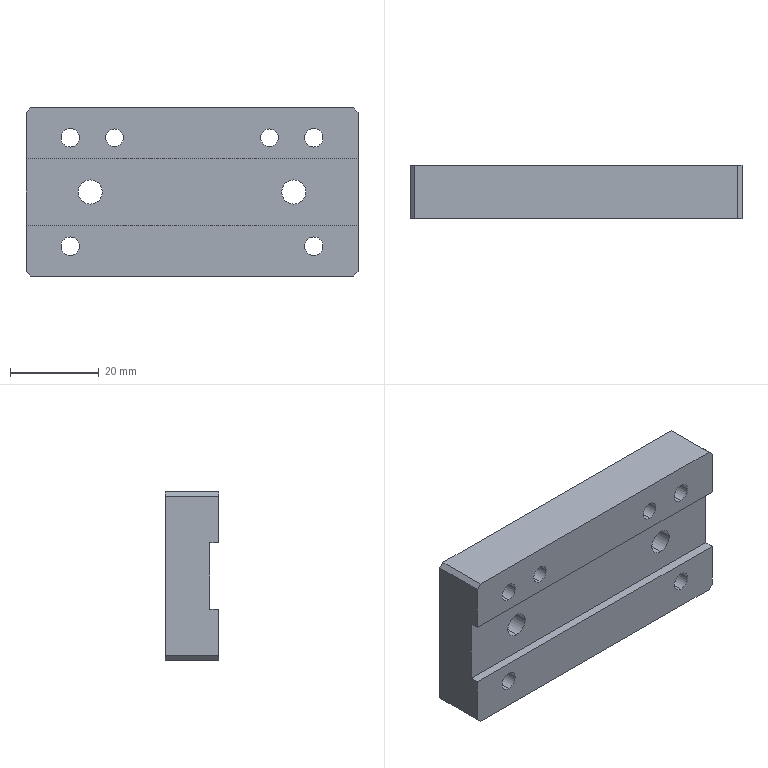Part | STEP file | 10000020593swp000-1 | 1 solid | 40 faces | box 75 x 12 x 38 mm | volume 29849 mm3 | cylinder 20 | plane 16 | cone 4 | commonest cylinder face diameters 4.2 x8 4 x4 5.5 x4 10 x4
STEP:
#1=CARTESIAN_POINT('',(-17.5,11.5,10.25));
#2=VERTEX_POINT('',#1);
#3=CARTESIAN_POINT('',(-17.5,11.5,14.25));
#4=VERTEX_POINT('',#3);
#5=CARTESIAN_POINT('',(-17.5,11.5,12.25));
#6=DIRECTION('',(0.,1.,0.));
#7=DIRECTION('',(0.,0.,1.));
#8=AXIS2_PLACEMENT_3D('',#5,#6,#7);
#9=CIRCLE('',#8,2.);
#10=EDGE_CURVE('',#2,#4,#9,.T.);
#11=ORIENTED_EDGE('',*,*,#10,.F.);
#12=CARTESIAN_POINT('',(-17.5,12.,9.75));
#13=VERTEX_POINT('',#12);
#14=CARTESIAN_POINT('',(-17.5,11.5,10.25));
#15=DIRECTION('',(0.,0.7071,-0.7071));
#16=VECTOR('',#15,1000.);
#17=LINE('',#14,#16);
#18=EDGE_CURVE('',#2,#13,#17,.T.);
#19=ORIENTED_EDGE('',*,*,#18,.T.);
#20=CARTESIAN_POINT('',(-17.5,12.,14.75));
#21=VERTEX_POINT('',#20);
#22=CARTESIAN_POINT('',(-17.5,12.,12.25));
#23=DIRECTION('',(0.,-1.,0.));
#24=DIRECTION('',(0.,0.,1.));
#25=AXIS2_PLACEMENT_3D('',#22,#23,#24);
#26=CIRCLE('',#25,2.5);
#27=EDGE_CURVE('',#21,#13,#26,.T.);
#28=ORIENTED_EDGE('',*,*,#27,.F.);
#29=CARTESIAN_POINT('',(-17.5,11.5,14.25));
#30=DIRECTION('',(0.,0.7071,0.7071));
#31=VECTOR('',#30,1000.);
#32=LINE('',#29,#31);
#33=EDGE_CURVE('',#4,#21,#32,.T.);
#34=ORIENTED_EDGE('',*,*,#33,.F.);
#35=EDGE_LOOP('',(#11,#19,#28,#34));
#36=FACE_OUTER_BOUND('',#35,.T.);
#37=CARTESIAN_POINT('',(-17.5,11.5,12.25));
#38=DIRECTION('',(0.,1.,0.));
#39=DIRECTION('',(0.,0.,1.));
#40=AXIS2_PLACEMENT_3D('',#37,#38,#39);
#41=CONICAL_SURFACE('',#40,2.,0.7854);
#42=ADVANCED_FACE('',(#36),#41,.F.);
#43=CARTESIAN_POINT('',(17.5,11.5,10.25));
#44=VERTEX_POINT('',#43);
#45=CARTESIAN_POINT('',(17.5,11.5,14.25));
#46=VERTEX_POINT('',#45);
#47=CARTESIAN_POINT('',(17.5,11.5,12.25));
#48=DIRECTION('',(0.,1.,0.));
#49=DIRECTION('',(0.,0.,1.));
#50=AXIS2_PLACEMENT_3D('',#47,#48,#49);
#51=CIRCLE('',#50,2.);
#52=EDGE_CURVE('',#44,#46,#51,.T.);
#53=ORIENTED_EDGE('',*,*,#52,.F.);
#54=CARTESIAN_POINT('',(17.5,12.,9.75));
#55=VERTEX_POINT('',#54);
#56=CARTESIAN_POINT('',(17.5,11.5,10.25));
#57=DIRECTION('',(0.,0.7071,-0.7071));
#58=VECTOR('',#57,1000.);
#59=LINE('',#56,#58);
#60=EDGE_CURVE('',#44,#55,#59,.T.);
#61=ORIENTED_EDGE('',*,*,#60,.T.);
#62=CARTESIAN_POINT('',(17.5,12.,14.75));
#63=VERTEX_POINT('',#62);
#64=CARTESIAN_POINT('',(17.5,12.,12.25));
#65=DIRECTION('',(0.,-1.,0.));
#66=DIRECTION('',(0.,0.,1.));
#67=AXIS2_PLACEMENT_3D('',#64,#65,#66);
#68=CIRCLE('',#67,2.5);
#69=EDGE_CURVE('',#63,#55,#68,.T.);
#70=ORIENTED_EDGE('',*,*,#69,.F.);
#71=CARTESIAN_POINT('',(17.5,11.5,14.25));
#72=DIRECTION('',(0.,0.7071,0.7071));
#73=VECTOR('',#72,1000.);
#74=LINE('',#71,#73);
#75=EDGE_CURVE('',#46,#63,#74,.T.);
#76=ORIENTED_EDGE('',*,*,#75,.F.);
#77=EDGE_LOOP('',(#53,#61,#70,#76));
#78=FACE_OUTER_BOUND('',#77,.T.);
#79=CARTESIAN_POINT('',(17.5,11.5,12.25));
#80=DIRECTION('',(0.,1.,0.));
#81=DIRECTION('',(0.,0.,1.));
#82=AXIS2_PLACEMENT_3D('',#79,#80,#81);
#83=CONICAL_SURFACE('',#82,2.,0.7854);
#84=ADVANCED_FACE('',(#78),#83,.F.);
#85=CARTESIAN_POINT('',(23.,6.3,-5.));
#86=VERTEX_POINT('',#85);
#87=CARTESIAN_POINT('',(23.,6.3,5.));
#88=VERTEX_POINT('',#87);
#89=CARTESIAN_POINT('',(23.,6.3,0.));
#90=DIRECTION('',(0.,1.,0.));
#91=DIRECTION('',(0.,0.,1.));
#92=AXIS2_PLACEMENT_3D('',#89,#90,#91);
#93=CIRCLE('',#92,5.);
#94=EDGE_CURVE('',#86,#88,#93,.T.);
#95=ORIENTED_EDGE('',*,*,#94,.F.);
#96=CARTESIAN_POINT('',(23.,12.,-5.));
#97=VERTEX_POINT('',#96);
#98=CARTESIAN_POINT('',(23.,12.,-5.));
#99=DIRECTION('',(0.,1.,0.));
#100=VECTOR('',#99,1000.);
#101=LINE('',#98,#100);
#102=EDGE_CURVE('',#86,#97,#101,.T.);
#103=ORIENTED_EDGE('',*,*,#102,.T.);
#104=CARTESIAN_POINT('',(23.,12.,5.));
#105=VERTEX_POINT('',#104);
#106=CARTESIAN_POINT('',(23.,12.,0.));
#107=DIRECTION('',(0.,1.,0.));
#108=DIRECTION('',(0.,0.,1.));
#109=AXIS2_PLACEMENT_3D('',#106,#107,#108);
#110=CIRCLE('',#109,5.);
#111=EDGE_CURVE('',#97,#105,#110,.T.);
#112=ORIENTED_EDGE('',*,*,#111,.T.);
#113=CARTESIAN_POINT('',(23.,12.,5.));
#114=DIRECTION('',(0.,1.,0.));
#115=VECTOR('',#114,1000.);
#116=LINE('',#113,#115);
#117=EDGE_CURVE('',#88,#105,#116,.T.);
#118=ORIENTED_EDGE('',*,*,#117,.F.);
#119=EDGE_LOOP('',(#95,#103,#112,#118));
#120=FACE_OUTER_BOUND('',#119,.T.);
#121=CARTESIAN_POINT('',(23.,12.,0.));
#122=DIRECTION('',(0.,1.,0.));
#123=DIRECTION('',(0.,0.,1.));
#124=AXIS2_PLACEMENT_3D('',#121,#122,#123);
#125=CYLINDRICAL_SURFACE('',#124,5.);
#126=ADVANCED_FACE('',(#120),#125,.F.);
#127=CARTESIAN_POINT('',(23.,2.,-2.75));
#128=VERTEX_POINT('',#127);
#129=CARTESIAN_POINT('',(23.,2.,2.75));
#130=VERTEX_POINT('',#129);
#131=CARTESIAN_POINT('',(23.,2.,0.));
#132=DIRECTION('',(0.,1.,0.));
#133=DIRECTION('',(0.,0.,1.));
#134=AXIS2_PLACEMENT_3D('',#131,#132,#133);
#135=CIRCLE('',#134,2.75);
#136=EDGE_CURVE('',#128,#130,#135,.T.);
#137=ORIENTED_EDGE('',*,*,#136,.F.);
#138=CARTESIAN_POINT('',(23.,6.3,-2.75));
#139=VERTEX_POINT('',#138);
#140=CARTESIAN_POINT('',(23.,12.,-2.75));
#141=DIRECTION('',(0.,1.,0.));
#142=VECTOR('',#141,1000.);
#143=LINE('',#140,#142);
#144=EDGE_CURVE('',#128,#139,#143,.T.);
#145=ORIENTED_EDGE('',*,*,#144,.T.);
#146=CARTESIAN_POINT('',(23.,6.3,2.75));
#147=VERTEX_POINT('',#146);
#148=CARTESIAN_POINT('',(23.,6.3,0.));
#149=DIRECTION('',(0.,1.,0.));
#150=DIRECTION('',(0.,0.,1.));
#151=AXIS2_PLACEMENT_3D('',#148,#149,#150);
#152=CIRCLE('',#151,2.75);
#153=EDGE_CURVE('',#139,#147,#152,.T.);
#154=ORIENTED_EDGE('',*,*,#153,.T.);
#155=CARTESIAN_POINT('',(23.,12.,2.75));
#156=DIRECTION('',(0.,1.,0.));
#157=VECTOR('',#156,1000.);
#158=LINE('',#155,#157);
#159=EDGE_CURVE('',#130,#147,#158,.T.);
#160=ORIENTED_EDGE('',*,*,#159,.F.);
#161=EDGE_LOOP('',(#137,#145,#154,#160));
#162=FACE_OUTER_BOUND('',#161,.T.);
#163=CARTESIAN_POINT('',(23.,12.,0.));
#164=DIRECTION('',(0.,1.,0.));
#165=DIRECTION('',(0.,0.,1.));
#166=AXIS2_PLACEMENT_3D('',#163,#164,#165);
#167=CYLINDRICAL_SURFACE('',#166,2.75);
#168=ADVANCED_FACE('',(#162),#167,.F.);
#169=CARTESIAN_POINT('',(-23.,6.3,-5.));
#170=VERTEX_POINT('',#169);
#171=CARTESIAN_POINT('',(-23.,6.3,5.));
#172=VERTEX_POINT('',#171);
#173=CARTESIAN_POINT('',(-23.,6.3,0.));
#174=DIRECTION('',(0.,1.,0.));
#175=DIRECTION('',(0.,0.,1.));
#176=AXIS2_PLACEMENT_3D('',#173,#174,#175);
#177=CIRCLE('',#176,5.);
#178=EDGE_CURVE('',#170,#172,#177,.T.);
#179=ORIENTED_EDGE('',*,*,#178,.F.);
#180=CARTESIAN_POINT('',(-23.,12.,-5.));
#181=VERTEX_POINT('',#180);
#182=CARTESIAN_POINT('',(-23.,12.,-5.));
#183=DIRECTION('',(0.,1.,0.));
#184=VECTOR('',#183,1000.);
#185=LINE('',#182,#184);
#186=EDGE_CURVE('',#170,#181,#185,.T.);
#187=ORIENTED_EDGE('',*,*,#186,.T.);
#188=CARTESIAN_POINT('',(-23.,12.,5.));
#189=VERTEX_POINT('',#188);
#190=CARTESIAN_POINT('',(-23.,12.,0.));
#191=DIRECTION('',(0.,1.,0.));
#192=DIRECTION('',(0.,0.,1.));
#193=AXIS2_PLACEMENT_3D('',#190,#191,#192);
#194=CIRCLE('',#193,5.);
#195=EDGE_CURVE('',#181,#189,#194,.T.);
#196=ORIENTED_EDGE('',*,*,#195,.T.);
#197=CARTESIAN_POINT('',(-23.,12.,5.));
#198=DIRECTION('',(0.,1.,0.));
#199=VECTOR('',#198,1000.);
#200=LINE('',#197,#199);
#201=EDGE_CURVE('',#172,#189,#200,.T.);
#202=ORIENTED_EDGE('',*,*,#201,.F.);
#203=EDGE_LOOP('',(#179,#187,#196,#202));
#204=FACE_OUTER_BOUND('',#203,.T.);
#205=CARTESIAN_POINT('',(-23.,12.,0.));
#206=DIRECTION('',(0.,1.,0.));
#207=DIRECTION('',(0.,0.,1.));
#208=AXIS2_PLACEMENT_3D('',#205,#206,#207);
#209=CYLINDRICAL_SURFACE('',#208,5.);
#210=ADVANCED_FACE('',(#204),#209,.F.);
#211=CARTESIAN_POINT('',(-23.,2.,-2.75));
#212=VERTEX_POINT('',#211);
#213=CARTESIAN_POINT('',(-23.,2.,2.75));
#214=VERTEX_POINT('',#213);
#215=CARTESIAN_POINT('',(-23.,2.,0.));
#216=DIRECTION('',(0.,1.,0.));
#217=DIRECTION('',(0.,0.,1.));
#218=AXIS2_PLACEMENT_3D('',#215,#216,#217);
#219=CIRCLE('',#218,2.75);
#220=EDGE_CURVE('',#212,#214,#219,.T.);
#221=ORIENTED_EDGE('',*,*,#220,.F.);
#222=CARTESIAN_POINT('',(-23.,6.3,-2.75));
#223=VERTEX_POINT('',#222);
#224=CARTESIAN_POINT('',(-23.,12.,-2.75));
#225=DIRECTION('',(0.,1.,0.));
#226=VECTOR('',#225,1000.);
#227=LINE('',#224,#226);
#228=EDGE_CURVE('',#212,#223,#227,.T.);
#229=ORIENTED_EDGE('',*,*,#228,.T.);
#230=CARTESIAN_POINT('',(-23.,6.3,2.75));
#231=VERTEX_POINT('',#230);
#232=CARTESIAN_POINT('',(-23.,6.3,0.));
#233=DIRECTION('',(0.,1.,0.));
#234=DIRECTION('',(0.,0.,1.));
#235=AXIS2_PLACEMENT_3D('',#232,#233,#234);
#236=CIRCLE('',#235,2.75);
#237=EDGE_CURVE('',#223,#231,#236,.T.);
#238=ORIENTED_EDGE('',*,*,#237,.T.);
#239=CARTESIAN_POINT('',(-23.,12.,2.75));
#240=DIRECTION('',(0.,1.,0.));
#241=VECTOR('',#240,1000.);
#242=LINE('',#239,#241);
#243=EDGE_CURVE('',#214,#231,#242,.T.);
#244=ORIENTED_EDGE('',*,*,#243,.F.);
#245=EDGE_LOOP('',(#221,#229,#238,#244));
#246=FACE_OUTER_BOUND('',#245,.T.);
#247=CARTESIAN_POINT('',(-23.,12.,0.));
#248=DIRECTION('',(0.,1.,0.));
#249=DIRECTION('',(0.,0.,1.));
#250=AXIS2_PLACEMENT_3D('',#247,#248,#249);
#251=CYLINDRICAL_SURFACE('',#250,2.75);
#252=ADVANCED_FACE('',(#246),#251,.F.);
#253=CARTESIAN_POINT('',(-17.5,0.,10.25));
#254=VERTEX_POINT('',#253);
#255=CARTESIAN_POINT('',(-17.5,0.,14.25));
#256=VERTEX_POINT('',#255);
#257=CARTESIAN_POINT('',(-17.5,0.,12.25));
#258=DIRECTION('',(0.,1.,0.));
#259=DIRECTION('',(0.,0.,1.));
#260=AXIS2_PLACEMENT_3D('',#257,#258,#259);
#261=CIRCLE('',#260,2.);
#262=EDGE_CURVE('',#254,#256,#261,.T.);
#263=ORIENTED_EDGE('',*,*,#262,.F.);
#264=CARTESIAN_POINT('',(-17.5,12.,10.25));
#265=DIRECTION('',(0.,1.,0.));
#266=VECTOR('',#265,1000.);
#267=LINE('',#264,#266);
#268=EDGE_CURVE('',#254,#2,#267,.T.);
#269=ORIENTED_EDGE('',*,*,#268,.T.);
#270=ORIENTED_EDGE('',*,*,#10,.T.);
#271=CARTESIAN_POINT('',(-17.5,12.,14.25));
#272=DIRECTION('',(0.,1.,0.));
#273=VECTOR('',#272,1000.);
#274=LINE('',#271,#273);
#275=EDGE_CURVE('',#256,#4,#274,.T.);
#276=ORIENTED_EDGE('',*,*,#275,.F.);
#277=EDGE_LOOP('',(#263,#269,#270,#276));
#278=FACE_OUTER_BOUND('',#277,.T.);
#279=CARTESIAN_POINT('',(-17.5,12.,12.25));
#280=DIRECTION('',(0.,1.,0.));
#281=DIRECTION('',(0.,0.,1.));
#282=AXIS2_PLACEMENT_3D('',#279,#280,#281);
#283=CYLINDRICAL_SURFACE('',#282,2.);
#284=ADVANCED_FACE('',(#278),#283,.F.);
#285=CARTESIAN_POINT('',(17.5,0.,10.25));
#286=VERTEX_POINT('',#285);
#287=CARTESIAN_POINT('',(17.5,0.,14.25));
#288=VERTEX_POINT('',#287);
#289=CARTESIAN_POINT('',(17.5,0.,12.25));
#290=DIRECTION('',(0.,1.,0.));
#291=DIRECTION('',(0.,0.,1.));
#292=AXIS2_PLACEMENT_3D('',#289,#290,#291);
#293=CIRCLE('',#292,2.);
#294=EDGE_CURVE('',#286,#288,#293,.T.);
#295=ORIENTED_EDGE('',*,*,#294,.F.);
#296=CARTESIAN_POINT('',(17.5,12.,10.25));
#297=DIRECTION('',(0.,1.,0.));
#298=VECTOR('',#297,1000.);
#299=LINE('',#296,#298);
#300=EDGE_CURVE('',#286,#44,#299,.T.);
#301=ORIENTED_EDGE('',*,*,#300,.T.);
#302=ORIENTED_EDGE('',*,*,#52,.T.);
#303=CARTESIAN_POINT('',(17.5,12.,14.25));
#304=DIRECTION('',(0.,1.,0.));
#305=VECTOR('',#304,1000.);
#306=LINE('',#303,#305);
#307=EDGE_CURVE('',#288,#46,#306,.T.);
#308=ORIENTED_EDGE('',*,*,#307,.F.);
#309=EDGE_LOOP('',(#295,#301,#302,#308));
#310=FACE_OUTER_BOUND('',#309,.T.);
#311=CARTESIAN_POINT('',(17.5,12.,12.25));
#312=DIRECTION('',(0.,1.,0.));
#313=DIRECTION('',(0.,0.,1.));
#314=AXIS2_PLACEMENT_3D('',#311,#312,#313);
#315=CYLINDRICAL_SURFACE('',#314,2.);
#316=ADVANCED_FACE('',(#310),#315,.F.);
#317=CARTESIAN_POINT('',(-27.5,0.,-14.35));
#318=VERTEX_POINT('',#317);
#319=CARTESIAN_POINT('',(-27.5,0.,-10.15));
#320=VERTEX_POINT('',#319);
#321=CARTESIAN_POINT('',(-27.5,0.,-12.25));
#322=DIRECTION('',(0.,1.,0.));
#323=DIRECTION('',(0.,0.,1.));
#324=AXIS2_PLACEMENT_3D('',#321,#322,#323);
#325=CIRCLE('',#324,2.1);
#326=EDGE_CURVE('',#318,#320,#325,.T.);
#327=ORIENTED_EDGE('',*,*,#326,.F.);
#328=CARTESIAN_POINT('',(-27.5,12.,-14.35));
#329=VERTEX_POINT('',#328);
#330=CARTESIAN_POINT('',(-27.5,12.,-14.35));
#331=DIRECTION('',(0.,1.,0.));
#332=VECTOR('',#331,1000.);
#333=LINE('',#330,#332);
#334=EDGE_CURVE('',#318,#329,#333,.T.);
#335=ORIENTED_EDGE('',*,*,#334,.T.);
#336=CARTESIAN_POINT('',(-27.5,12.,-10.15));
#337=VERTEX_POINT('',#336);
#338=CARTESIAN_POINT('',(-27.5,12.,-12.25));
#339=DIRECTION('',(0.,1.,0.));
#340=DIRECTION('',(0.,0.,1.));
#341=AXIS2_PLACEMENT_3D('',#338,#339,#340);
#342=CIRCLE('',#341,2.1);
#343=EDGE_CURVE('',#329,#337,#342,.T.);
#344=ORIENTED_EDGE('',*,*,#343,.T.);
#345=CARTESIAN_POINT('',(-27.5,12.,-10.15));
#346=DIRECTION('',(0.,1.,0.));
#347=VECTOR('',#346,1000.);
#348=LINE('',#345,#347);
#349=EDGE_CURVE('',#320,#337,#348,.T.);
#350=ORIENTED_EDGE('',*,*,#349,.F.);
#351=EDGE_LOOP('',(#327,#335,#344,#350));
#352=FACE_OUTER_BOUND('',#351,.T.);
#353=CARTESIAN_POINT('',(-27.5,12.,-12.25));
#354=DIRECTION('',(0.,1.,0.));
#355=DIRECTION('',(0.,0.,1.));
#356=AXIS2_PLACEMENT_3D('',#353,#354,#355);
#357=CYLINDRICAL_SURFACE('',#356,2.1);
#358=ADVANCED_FACE('',(#352),#357,.F.);
#359=CARTESIAN_POINT('',(-27.5,0.,10.15));
#360=VERTEX_POINT('',#359);
#361=CARTESIAN_POINT('',(-27.5,0.,14.35));
#362=VERTEX_POINT('',#361);
#363=CARTESIAN_POINT('',(-27.5,0.,12.25));
#364=DIRECTION('',(0.,1.,0.));
#365=DIRECTION('',(0.,0.,1.));
#366=AXIS2_PLACEMENT_3D('',#363,#364,#365);
#367=CIRCLE('',#366,2.1);
#368=EDGE_CURVE('',#360,#362,#367,.T.);
#369=ORIENTED_EDGE('',*,*,#368,.F.);
#370=CARTESIAN_POINT('',(-27.5,12.,10.15));
#371=VERTEX_POINT('',#370);
#372=CARTESIAN_POINT('',(-27.5,12.,10.15));
#373=DIRECTION('',(0.,1.,0.));
#374=VECTOR('',#373,1000.);
#375=LINE('',#372,#374);
#376=EDGE_CURVE('',#360,#371,#375,.T.);
#377=ORIENTED_EDGE('',*,*,#376,.T.);
#378=CARTESIAN_POINT('',(-27.5,12.,14.35));
#379=VERTEX_POINT('',#378);
#380=CARTESIAN_POINT('',(-27.5,12.,12.25));
#381=DIRECTION('',(0.,1.,0.));
#382=DIRECTION('',(0.,0.,1.));
#383=AXIS2_PLACEMENT_3D('',#380,#381,#382);
#384=CIRCLE('',#383,2.1);
#385=EDGE_CURVE('',#371,#379,#384,.T.);
#386=ORIENTED_EDGE('',*,*,#385,.T.);
#387=CARTESIAN_POINT('',(-27.5,12.,14.35));
#388=DIRECTION('',(0.,1.,0.));
#389=VECTOR('',#388,1000.);
#390=LINE('',#387,#389);
#391=EDGE_CURVE('',#362,#379,#390,.T.);
#392=ORIENTED_EDGE('',*,*,#391,.F.);
#393=EDGE_LOOP('',(#369,#377,#386,#392));
#394=FACE_OUTER_BOUND('',#393,.T.);
#395=CARTESIAN_POINT('',(-27.5,12.,12.25));
#396=DIRECTION('',(0.,1.,0.));
#397=DIRECTION('',(0.,0.,1.));
#398=AXIS2_PLACEMENT_3D('',#395,#396,#397);
#399=CYLINDRICAL_SURFACE('',#398,2.1);
#400=ADVANCED_FACE('',(#394),#399,.F.);
#401=CARTESIAN_POINT('',(27.5,0.,10.15));
#402=VERTEX_POINT('',#401);
#403=CARTESIAN_POINT('',(27.5,0.,14.35));
#404=VERTEX_POINT('',#403);
#405=CARTESIAN_POINT('',(27.5,0.,12.25));
#406=DIRECTION('',(0.,1.,0.));
#407=DIRECTION('',(0.,0.,1.));
#408=AXIS2_PLACEMENT_3D('',#405,#406,#407);
#409=CIRCLE('',#408,2.1);
#410=EDGE_CURVE('',#402,#404,#409,.T.);
#411=ORIENTED_EDGE('',*,*,#410,.F.);
#412=CARTESIAN_POINT('',(27.5,12.,10.15));
#413=VERTEX_POINT('',#412);
#414=CARTESIAN_POINT('',(27.5,12.,10.15));
#415=DIRECTION('',(0.,1.,0.));
#416=VECTOR('',#415,1000.);
#417=LINE('',#414,#416);
#418=EDGE_CURVE('',#402,#413,#417,.T.);
#419=ORIENTED_EDGE('',*,*,#418,.T.);
#420=CARTESIAN_POINT('',(27.5,12.,14.35));
#421=VERTEX_POINT('',#420);
#422=CARTESIAN_POINT('',(27.5,12.,12.25));
#423=DIRECTION('',(0.,1.,0.));
#424=DIRECTION('',(0.,0.,1.));
#425=AXIS2_PLACEMENT_3D('',#422,#423,#424);
#426=CIRCLE('',#425,2.1);
#427=EDGE_CURVE('',#413,#421,#426,.T.);
#428=ORIENTED_EDGE('',*,*,#427,.T.);
#429=CARTESIAN_POINT('',(27.5,12.,14.35));
#430=DIRECTION('',(0.,1.,0.));
#431=VECTOR('',#430,1000.);
#432=LINE('',#429,#431);
#433=EDGE_CURVE('',#404,#421,#432,.T.);
#434=ORIENTED_EDGE('',*,*,#433,.F.);
#435=EDGE_LOOP('',(#411,#419,#428,#434));
#436=FACE_OUTER_BOUND('',#435,.T.);
#437=CARTESIAN_POINT('',(27.5,12.,12.25));
#438=DIRECTION('',(0.,1.,0.));
#439=DIRECTION('',(0.,0.,1.));
#440=AXIS2_PLACEMENT_3D('',#437,#438,#439);
#441=CYLINDRICAL_SURFACE('',#440,2.1);
#442=ADVANCED_FACE('',(#436),#441,.F.);
#443=CARTESIAN_POINT('',(27.5,0.,-14.35));
#444=VERTEX_POINT('',#443);
#445=CARTESIAN_POINT('',(27.5,0.,-10.15));
#446=VERTEX_POINT('',#445);
#447=CARTESIAN_POINT('',(27.5,0.,-12.25));
#448=DIRECTION('',(0.,1.,0.));
#449=DIRECTION('',(0.,0.,1.));
#450=AXIS2_PLACEMENT_3D('',#447,#448,#449);
#451=CIRCLE('',#450,2.1);
#452=EDGE_CURVE('',#444,#446,#451,.T.);
#453=ORIENTED_EDGE('',*,*,#452,.F.);
#454=CARTESIAN_POINT('',(27.5,12.,-14.35));
#455=VERTEX_POINT('',#454);
#456=CARTESIAN_POINT('',(27.5,12.,-14.35));
#457=DIRECTION('',(0.,1.,0.));
#458=VECTOR('',#457,1000.);
#459=LINE('',#456,#458);
#460=EDGE_CURVE('',#444,#455,#459,.T.);
#461=ORIENTED_EDGE('',*,*,#460,.T.);
#462=CARTESIAN_POINT('',(27.5,12.,-10.15));
#463=VERTEX_POINT('',#462);
#464=CARTESIAN_POINT('',(27.5,12.,-12.25));
#465=DIRECTION('',(0.,1.,0.));
#466=DIRECTION('',(0.,0.,1.));
#467=AXIS2_PLACEMENT_3D('',#464,#465,#466);
#468=CIRCLE('',#467,2.1);
#469=EDGE_CURVE('',#455,#463,#468,.T.);
#470=ORIENTED_EDGE('',*,*,#469,.T.);
#471=CARTESIAN_POINT('',(27.5,12.,-10.15));
#472=DIRECTION('',(0.,1.,0.));
#473=VECTOR('',#472,1000.);
#474=LINE('',#471,#473);
#475=EDGE_CURVE('',#446,#463,#474,.T.);
#476=ORIENTED_EDGE('',*,*,#475,.F.);
#477=EDGE_LOOP('',(#453,#461,#470,#476));
#478=FACE_OUTER_BOUND('',#477,.T.);
#479=CARTESIAN_POINT('',(27.5,12.,-12.25));
#480=DIRECTION('',(0.,1.,0.));
#481=DIRECTION('',(0.,0.,1.));
#482=AXIS2_PLACEMENT_3D('',#479,#480,#481);
#483=CYLINDRICAL_SURFACE('',#482,2.1);
#484=ADVANCED_FACE('',(#478),#483,.F.);
#485=CARTESIAN_POINT('',(27.5,0.,-12.25));
#486=DIRECTION('',(0.,1.,0.));
#487=DIRECTION('',(0.,0.,1.));
#488=AXIS2_PLACEMENT_3D('',#485,#486,#487);
#489=CIRCLE('',#488,2.1);
#490=EDGE_CURVE('',#446,#444,#489,.T.);
#491=ORIENTED_EDGE('',*,*,#490,.T.);
#492=ORIENTED_EDGE('',*,*,#452,.T.);
#493=EDGE_LOOP('',(#491,#492));
#494=FACE_BOUND('',#493,.T.);
#495=CARTESIAN_POINT('',(-27.5,0.,-12.25));
#496=DIRECTION('',(0.,1.,0.));
#497=DIRECTION('',(0.,0.,1.));
#498=AXIS2_PLACEMENT_3D('',#495,#496,#497);
#499=CIRCLE('',#498,2.1);
#500=EDGE_CURVE('',#320,#318,#499,.T.);
#501=ORIENTED_EDGE('',*,*,#500,.T.);
#502=ORIENTED_EDGE('',*,*,#326,.T.);
#503=EDGE_LOOP('',(#501,#502));
#504=FACE_BOUND('',#503,.T.);
#505=CARTESIAN_POINT('',(36.5,0.,-19.));
#506=VERTEX_POINT('',#505);
#507=CARTESIAN_POINT('',(-36.5,0.,-19.));
#508=VERTEX_POINT('',#507);
#509=CARTESIAN_POINT('',(-37.5,0.,-19.));
#510=DIRECTION('',(-1.,0.,0.));
#511=VECTOR('',#510,1000.);
#512=LINE('',#509,#511);
#513=EDGE_CURVE('',#506,#508,#512,.T.);
#514=ORIENTED_EDGE('',*,*,#513,.F.);
#515=CARTESIAN_POINT('',(37.5,0.,-18.));
#516=VERTEX_POINT('',#515);
#517=CARTESIAN_POINT('',(36.5,0.,-19.));
#518=DIRECTION('',(0.7071,0.,0.7071));
#519=VECTOR('',#518,1000.);
#520=LINE('',#517,#519);
#521=EDGE_CURVE('',#506,#516,#520,.T.);
#522=ORIENTED_EDGE('',*,*,#521,.T.);
#523=CARTESIAN_POINT('',(37.5,0.,-7.525));
#524=VERTEX_POINT('',#523);
#525=CARTESIAN_POINT('',(37.5,0.,-19.));
#526=DIRECTION('',(0.,0.,-1.));
#527=VECTOR('',#526,1000.);
#528=LINE('',#525,#527);
#529=EDGE_CURVE('',#524,#516,#528,.T.);
#530=ORIENTED_EDGE('',*,*,#529,.F.);
#531=CARTESIAN_POINT('',(-37.5,0.,-7.525));
#532=VERTEX_POINT('',#531);
#533=CARTESIAN_POINT('',(-37.5,0.,-7.525));
#534=DIRECTION('',(1.,0.,0.));
#535=VECTOR('',#534,1000.);
#536=LINE('',#533,#535);
#537=EDGE_CURVE('',#532,#524,#536,.T.);
#538=ORIENTED_EDGE('',*,*,#537,.F.);
#539=CARTESIAN_POINT('',(-37.5,0.,-18.));
#540=VERTEX_POINT('',#539);
#541=CARTESIAN_POINT('',(-37.5,0.,-19.));
#542=DIRECTION('',(0.,0.,1.));
#543=VECTOR('',#542,1000.);
#544=LINE('',#541,#543);
#545=EDGE_CURVE('',#540,#532,#544,.T.);
#546=ORIENTED_EDGE('',*,*,#545,.F.);
#547=CARTESIAN_POINT('',(-37.5,0.,-18.));
#548=DIRECTION('',(0.7071,0.,-0.7071));
#549=VECTOR('',#548,1000.);
#550=LINE('',#547,#549);
#551=EDGE_CURVE('',#540,#508,#550,.T.);
#552=ORIENTED_EDGE('',*,*,#551,.T.);
#553=EDGE_LOOP('',(#514,#522,#530,#538,#546,#552));
#554=FACE_OUTER_BOUND('',#553,.T.);
#555=CARTESIAN_POINT('',(0.,0.,0.));
#556=DIRECTION('',(0.,1.,0.));
#557=DIRECTION('',(0.,0.,1.));
#558=AXIS2_PLACEMENT_3D('',#555,#556,#557);
#559=PLANE('',#558);
#560=ADVANCED_FACE('',(#494,#504,#554),#559,.F.);
#561=ORIENTED_EDGE('',*,*,#529,.T.);
#562=CARTESIAN_POINT('',(37.5,12.,-18.));
#563=VERTEX_POINT('',#562);
#564=CARTESIAN_POINT('',(37.5,12.,-18.));
#565=DIRECTION('',(0.,1.,0.));
#566=VECTOR('',#565,1000.);
#567=LINE('',#564,#566);
#568=EDGE_CURVE('',#516,#563,#567,.T.);
#569=ORIENTED_EDGE('',*,*,#568,.T.);
#570=CARTESIAN_POINT('',(37.5,12.,18.));
#571=VERTEX_POINT('',#570);
#572=CARTESIAN_POINT('',(37.5,12.,-19.));
#573=DIRECTION('',(0.,0.,-1.));
#574=VECTOR('',#573,1000.);
#575=LINE('',#572,#574);
#576=EDGE_CURVE('',#571,#563,#575,.T.);
#577=ORIENTED_EDGE('',*,*,#576,.F.);
#578=CARTESIAN_POINT('',(37.5,0.,18.));
#579=VERTEX_POINT('',#578);
#580=CARTESIAN_POINT('',(37.5,12.,18.));
#581=DIRECTION('',(0.,-1.,0.));
#582=VECTOR('',#581,1000.);
#583=LINE('',#580,#582);
#584=EDGE_CURVE('',#571,#579,#583,.T.);
#585=ORIENTED_EDGE('',*,*,#584,.T.);
#586=CARTESIAN_POINT('',(37.5,0.,7.525));
#587=VERTEX_POINT('',#586);
#588=CARTESIAN_POINT('',(37.5,0.,-19.));
#589=DIRECTION('',(0.,0.,-1.));
#590=VECTOR('',#589,1000.);
#591=LINE('',#588,#590);
#592=EDGE_CURVE('',#579,#587,#591,.T.);
#593=ORIENTED_EDGE('',*,*,#592,.T.);
#594=CARTESIAN_POINT('',(37.5,2.,7.525));
#595=VERTEX_POINT('',#594);
#596=CARTESIAN_POINT('',(37.5,2.,7.525));
#597=DIRECTION('',(0.,-1.,0.));
#598=VECTOR('',#597,1000.);
#599=LINE('',#596,#598);
#600=EDGE_CURVE('',#595,#587,#599,.T.);
#601=ORIENTED_EDGE('',*,*,#600,.F.);
#602=CARTESIAN_POINT('',(37.5,2.,-7.525));
#603=VERTEX_POINT('',#602);
#604=CARTESIAN_POINT('',(37.5,2.,-7.525));
#605=DIRECTION('',(0.,0.,1.));
#606=VECTOR('',#605,1000.);
#607=LINE('',#604,#606);
#608=EDGE_CURVE('',#603,#595,#607,.T.);
#609=ORIENTED_EDGE('',*,*,#608,.F.);
#610=CARTESIAN_POINT('',(37.5,2.,-7.525));
#611=DIRECTION('',(0.,-1.,0.));
#612=VECTOR('',#611,1000.);
#613=LINE('',#610,#612);
#614=EDGE_CURVE('',#603,#524,#613,.T.);
#615=ORIENTED_EDGE('',*,*,#614,.T.);
#616=EDGE_LOOP('',(#561,#569,#577,#585,#593,#601,#609,#615));
#617=FACE_OUTER_BOUND('',#616,.T.);
#618=CARTESIAN_POINT('',(37.5,12.,-19.));
#619=DIRECTION('',(-1.,0.,0.));
#620=DIRECTION('',(0.,0.,1.));
#621=AXIS2_PLACEMENT_3D('',#618,#619,#620);
#622=PLANE('',#621);
#623=ADVANCED_FACE('',(#617),#622,.F.);
#624=CARTESIAN_POINT('',(36.5,12.,-19.));
#625=VERTEX_POINT('',#624);
#626=CARTESIAN_POINT('',(-36.5,12.,-19.));
#627=VERTEX_POINT('',#626);
#628=CARTESIAN_POINT('',(-37.5,12.,-19.));
#629=DIRECTION('',(-1.,0.,0.));
#630=VECTOR('',#629,1000.);
#631=LINE('',#628,#630);
#632=EDGE_CURVE('',#625,#627,#631,.T.);
#633=ORIENTED_EDGE('',*,*,#632,.F.);
#634=CARTESIAN_POINT('',(36.5,12.,-19.));
#635=DIRECTION('',(0.,-1.,0.));
#636=VECTOR('',#635,1000.);
#637=LINE('',#634,#636);
#638=EDGE_CURVE('',#625,#506,#637,.T.);
#639=ORIENTED_EDGE('',*,*,#638,.T.);
#640=ORIENTED_EDGE('',*,*,#513,.T.);
#641=CARTESIAN_POINT('',(-36.5,12.,-19.));
#642=DIRECTION('',(0.,1.,0.));
#643=VECTOR('',#642,1000.);
#644=LINE('',#641,#643);
#645=EDGE_CURVE('',#508,#627,#644,.T.);
#646=ORIENTED_EDGE('',*,*,#645,.T.);
#647=EDGE_LOOP('',(#633,#639,#640,#646));
#648=FACE_OUTER_BOUND('',#647,.T.);
#649=CARTESIAN_POINT('',(-37.5,12.,-19.));
#650=DIRECTION('',(0.,0.,1.));
#651=DIRECTION('',(1.,0.,0.));
#652=AXIS2_PLACEMENT_3D('',#649,#650,#651);
#653=PLANE('',#652);
#654=ADVANCED_FACE('',(#648),#653,.F.);
#655=CARTESIAN_POINT('',(-37.5,0.,7.525));
#656=VERTEX_POINT('',#655);
#657=CARTESIAN_POINT('',(-37.5,0.,18.));
#658=VERTEX_POINT('',#657);
#659=CARTESIAN_POINT('',(-37.5,0.,-19.));
#660=DIRECTION('',(0.,0.,1.));
#661=VECTOR('',#660,1000.);
#662=LINE('',#659,#661);
#663=EDGE_CURVE('',#656,#658,#662,.T.);
#664=ORIENTED_EDGE('',*,*,#663,.T.);
#665=CARTESIAN_POINT('',(-37.5,12.,18.));
#666=VERTEX_POINT('',#665);
#667=CARTESIAN_POINT('',(-37.5,12.,18.));
#668=DIRECTION('',(0.,1.,0.));
#669=VECTOR('',#668,1000.);
#670=LINE('',#667,#669);
#671=EDGE_CURVE('',#658,#666,#670,.T.);
#672=ORIENTED_EDGE('',*,*,#671,.T.);
#673=CARTESIAN_POINT('',(-37.5,12.,-18.));
#674=VERTEX_POINT('',#673);
#675=CARTESIAN_POINT('',(-37.5,12.,-19.));
#676=DIRECTION('',(0.,0.,1.));
#677=VECTOR('',#676,1000.);
#678=LINE('',#675,#677);
#679=EDGE_CURVE('',#674,#666,#678,.T.);
#680=ORIENTED_EDGE('',*,*,#679,.F.);
#681=CARTESIAN_POINT('',(-37.5,12.,-18.));
#682=DIRECTION('',(0.,-1.,0.));
#683=VECTOR('',#682,1000.);
#684=LINE('',#681,#683);
#685=EDGE_CURVE('',#674,#540,#684,.T.);
#686=ORIENTED_EDGE('',*,*,#685,.T.);
#687=ORIENTED_EDGE('',*,*,#545,.T.);
#688=CARTESIAN_POINT('',(-37.5,2.,-7.525));
#689=VERTEX_POINT('',#688);
#690=CARTESIAN_POINT('',(-37.5,2.,-7.525));
#691=DIRECTION('',(0.,-1.,0.));
#692=VECTOR('',#691,1000.);
#693=LINE('',#690,#692);
#694=EDGE_CURVE('',#689,#532,#693,.T.);
#695=ORIENTED_EDGE('',*,*,#694,.F.);
#696=CARTESIAN_POINT('',(-37.5,2.,7.525));
#697=VERTEX_POINT('',#696);
#698=CARTESIAN_POINT('',(-37.5,2.,-7.525));
#699=DIRECTION('',(0.,0.,-1.));
#700=VECTOR('',#699,1000.);
#701=LINE('',#698,#700);
#702=EDGE_CURVE('',#697,#689,#701,.T.);
#703=ORIENTED_EDGE('',*,*,#702,.F.);
#704=CARTESIAN_POINT('',(-37.5,2.,7.525));
#705=DIRECTION('',(0.,-1.,0.));
#706=VECTOR('',#705,1000.);
#707=LINE('',#704,#706);
#708=EDGE_CURVE('',#697,#656,#707,.T.);
#709=ORIENTED_EDGE('',*,*,#708,.T.);
#710=EDGE_LOOP('',(#664,#672,#680,#686,#687,#695,#703,#709));
#711=FACE_OUTER_BOUND('',#710,.T.);
#712=CARTESIAN_POINT('',(-37.5,12.,-19.));
#713=DIRECTION('',(1.,0.,0.));
#714=DIRECTION('',(0.,0.,-1.));
#715=AXIS2_PLACEMENT_3D('',#712,#713,#714);
#716=PLANE('',#715);
#717=ADVANCED_FACE('',(#711),#716,.F.);
#718=CARTESIAN_POINT('',(-36.5,0.,19.));
#719=VERTEX_POINT('',#718);
#720=CARTESIAN_POINT('',(36.5,0.,19.));
#721=VERTEX_POINT('',#720);
#722=CARTESIAN_POINT('',(-37.5,0.,19.));
#723=DIRECTION('',(1.,0.,0.));
#724=VECTOR('',#723,1000.);
#725=LINE('',#722,#724);
#726=EDGE_CURVE('',#719,#721,#725,.T.);
#727=ORIENTED_EDGE('',*,*,#726,.T.);
#728=CARTESIAN_POINT('',(36.5,12.,19.));
#729=VERTEX_POINT('',#728);
#730=CARTESIAN_POINT('',(36.5,12.,19.));
#731=DIRECTION('',(0.,1.,0.));
#732=VECTOR('',#731,1000.);
#733=LINE('',#730,#732);
#734=EDGE_CURVE('',#721,#729,#733,.T.);
#735=ORIENTED_EDGE('',*,*,#734,.T.);
#736=CARTESIAN_POINT('',(-36.5,12.,19.));
#737=VERTEX_POINT('',#736);
#738=CARTESIAN_POINT('',(-37.5,12.,19.));
#739=DIRECTION('',(1.,0.,0.));
#740=VECTOR('',#739,1000.);
#741=LINE('',#738,#740);
#742=EDGE_CURVE('',#737,#729,#741,.T.);
#743=ORIENTED_EDGE('',*,*,#742,.F.);
#744=CARTESIAN_POINT('',(-36.5,12.,19.));
#745=DIRECTION('',(0.,-1.,0.));
#746=VECTOR('',#745,1000.);
#747=LINE('',#744,#746);
#748=EDGE_CURVE('',#737,#719,#747,.T.);
#749=ORIENTED_EDGE('',*,*,#748,.T.);
#750=EDGE_LOOP('',(#727,#735,#743,#749));
#751=FACE_OUTER_BOUND('',#750,.T.);
#752=CARTESIAN_POINT('',(-37.5,12.,19.));
#753=DIRECTION('',(0.,0.,-1.));
#754=DIRECTION('',(-1.,0.,0.));
#755=AXIS2_PLACEMENT_3D('',#752,#753,#754);
#756=PLANE('',#755);
#757=ADVANCED_FACE('',(#751),#756,.F.);
#758=ORIENTED_EDGE('',*,*,#69,.T.);
#759=CARTESIAN_POINT('',(17.5,12.,12.25));
#760=DIRECTION('',(0.,-1.,0.));
#761=DIRECTION('',(0.,0.,1.));
#762=AXIS2_PLACEMENT_3D('',#759,#760,#761);
#763=CIRCLE('',#762,2.5);
#764=EDGE_CURVE('',#55,#63,#763,.T.);
#765=ORIENTED_EDGE('',*,*,#764,.T.);
#766=EDGE_LOOP('',(#758,#765));
#767=FACE_BOUND('',#766,.T.);
#768=ORIENTED_EDGE('',*,*,#27,.T.);
#769=CARTESIAN_POINT('',(-17.5,12.,12.25));
#770=DIRECTION('',(0.,-1.,0.));
#771=DIRECTION('',(0.,0.,1.));
#772=AXIS2_PLACEMENT_3D('',#769,#770,#771);
#773=CIRCLE('',#772,2.5);
#774=EDGE_CURVE('',#13,#21,#773,.T.);
#775=ORIENTED_EDGE('',*,*,#774,.T.);
#776=EDGE_LOOP('',(#768,#775));
#777=FACE_BOUND('',#776,.T.);
#778=CARTESIAN_POINT('',(23.,12.,0.));
#779=DIRECTION('',(0.,1.,0.));
#780=DIRECTION('',(0.,0.,1.));
#781=AXIS2_PLACEMENT_3D('',#778,#779,#780);
#782=CIRCLE('',#781,5.);
#783=EDGE_CURVE('',#105,#97,#782,.T.);
#784=ORIENTED_EDGE('',*,*,#783,.F.);
#785=ORIENTED_EDGE('',*,*,#111,.F.);
#786=EDGE_LOOP('',(#784,#785));
#787=FACE_BOUND('',#786,.T.);
#788=CARTESIAN_POINT('',(-23.,12.,0.));
#789=DIRECTION('',(0.,1.,0.));
#790=DIRECTION('',(0.,0.,1.));
#791=AXIS2_PLACEMENT_3D('',#788,#789,#790);
#792=CIRCLE('',#791,5.);
#793=EDGE_CURVE('',#189,#181,#792,.T.);
#794=ORIENTED_EDGE('',*,*,#793,.F.);
#795=ORIENTED_EDGE('',*,*,#195,.F.);
#796=EDGE_LOOP('',(#794,#795));
#797=FACE_BOUND('',#796,.T.);
#798=CARTESIAN_POINT('',(-27.5,12.,-12.25));
#799=DIRECTION('',(0.,1.,0.));
#800=DIRECTION('',(0.,0.,1.));
#801=AXIS2_PLACEMENT_3D('',#798,#799,#800);
#802=CIRCLE('',#801,2.1);
#803=EDGE_CURVE('',#337,#329,#802,.T.);
#804=ORIENTED_EDGE('',*,*,#803,.F.);
#805=ORIENTED_EDGE('',*,*,#343,.F.);
#806=EDGE_LOOP('',(#804,#805));
#807=FACE_BOUND('',#806,.T.);
#808=CARTESIAN_POINT('',(-27.5,12.,12.25));
#809=DIRECTION('',(0.,1.,0.));
#810=DIRECTION('',(0.,0.,1.));
#811=AXIS2_PLACEMENT_3D('',#808,#809,#810);
#812=CIRCLE('',#811,2.1);
#813=EDGE_CURVE('',#379,#371,#812,.T.);
#814=ORIENTED_EDGE('',*,*,#813,.F.);
#815=ORIENTED_EDGE('',*,*,#385,.F.);
#816=EDGE_LOOP('',(#814,#815));
#817=FACE_BOUND('',#816,.T.);
#818=CARTESIAN_POINT('',(27.5,12.,12.25));
#819=DIRECTION('',(0.,1.,0.));
#820=DIRECTION('',(0.,0.,1.));
#821=AXIS2_PLACEMENT_3D('',#818,#819,#820);
#822=CIRCLE('',#821,2.1);
#823=EDGE_CURVE('',#421,#413,#822,.T.);
#824=ORIENTED_EDGE('',*,*,#823,.F.);
#825=ORIENTED_EDGE('',*,*,#427,.F.);
#826=EDGE_LOOP('',(#824,#825));
#827=FACE_BOUND('',#826,.T.);
#828=CARTESIAN_POINT('',(27.5,12.,-12.25));
#829=DIRECTION('',(0.,1.,0.));
#830=DIRECTION('',(0.,0.,1.));
#831=AXIS2_PLACEMENT_3D('',#828,#829,#830);
#832=CIRCLE('',#831,2.1);
#833=EDGE_CURVE('',#463,#455,#832,.T.);
#834=ORIENTED_EDGE('',*,*,#833,.F.);
#835=ORIENTED_EDGE('',*,*,#469,.F.);
#836=EDGE_LOOP('',(#834,#835));
#837=FACE_BOUND('',#836,.T.);
#838=ORIENTED_EDGE('',*,*,#576,.T.);
#839=CARTESIAN_POINT('',(27.75,12.,-27.75));
#840=DIRECTION('',(-0.7071,0.,-0.7071));
#841=VECTOR('',#840,1000.);
#842=LINE('',#839,#841);
#843=EDGE_CURVE('',#563,#625,#842,.T.);
#844=ORIENTED_EDGE('',*,*,#843,.T.);
#845=ORIENTED_EDGE('',*,*,#632,.T.);
#846=CARTESIAN_POINT('',(-27.75,12.,-27.75));
#847=DIRECTION('',(-0.7071,0.,0.7071));
#848=VECTOR('',#847,1000.);
#849=LINE('',#846,#848);
#850=EDGE_CURVE('',#627,#674,#849,.T.);
#851=ORIENTED_EDGE('',*,*,#850,.T.);
#852=ORIENTED_EDGE('',*,*,#679,.T.);
#853=CARTESIAN_POINT('',(-27.75,12.,27.75));
#854=DIRECTION('',(0.7071,0.,0.7071));
#855=VECTOR('',#854,1000.);
#856=LINE('',#853,#855);
#857=EDGE_CURVE('',#666,#737,#856,.T.);
#858=ORIENTED_EDGE('',*,*,#857,.T.);
#859=ORIENTED_EDGE('',*,*,#742,.T.);
#860=CARTESIAN_POINT('',(27.75,12.,27.75));
#861=DIRECTION('',(0.7071,0.,-0.7071));
#862=VECTOR('',#861,1000.);
#863=LINE('',#860,#862);
#864=EDGE_CURVE('',#729,#571,#863,.T.);
#865=ORIENTED_EDGE('',*,*,#864,.T.);
#866=EDGE_LOOP('',(#838,#844,#845,#851,#852,#858,#859,#865));
#867=FACE_OUTER_BOUND('',#866,.T.);
#868=CARTESIAN_POINT('',(0.,12.,0.));
#869=DIRECTION('',(0.,1.,0.));
#870=DIRECTION('',(0.,0.,1.));
#871=AXIS2_PLACEMENT_3D('',#868,#869,#870);
#872=PLANE('',#871);
#873=ADVANCED_FACE('',(#767,#777,#787,#797,#807,#817,#827,#837,#867),#872,.T.);
#874=CARTESIAN_POINT('',(-17.5,0.,12.25));
#875=DIRECTION('',(0.,1.,0.));
#876=DIRECTION('',(0.,0.,1.));
#877=AXIS2_PLACEMENT_3D('',#874,#875,#876);
#878=CIRCLE('',#877,2.);
#879=EDGE_CURVE('',#256,#254,#878,.T.);
#880=ORIENTED_EDGE('',*,*,#879,.T.);
#881=ORIENTED_EDGE('',*,*,#262,.T.);
#882=EDGE_LOOP('',(#880,#881));
#883=FACE_BOUND('',#882,.T.);
#884=CARTESIAN_POINT('',(17.5,0.,12.25));
#885=DIRECTION('',(0.,1.,0.));
#886=DIRECTION('',(0.,0.,1.));
#887=AXIS2_PLACEMENT_3D('',#884,#885,#886);
#888=CIRCLE('',#887,2.);
#889=EDGE_CURVE('',#288,#286,#888,.T.);
#890=ORIENTED_EDGE('',*,*,#889,.T.);
#891=ORIENTED_EDGE('',*,*,#294,.T.);
#892=EDGE_LOOP('',(#890,#891));
#893=FACE_BOUND('',#892,.T.);
#894=CARTESIAN_POINT('',(-27.5,0.,12.25));
#895=DIRECTION('',(0.,1.,0.));
#896=DIRECTION('',(0.,0.,1.));
#897=AXIS2_PLACEMENT_3D('',#894,#895,#896);
#898=CIRCLE('',#897,2.1);
#899=EDGE_CURVE('',#362,#360,#898,.T.);
#900=ORIENTED_EDGE('',*,*,#899,.T.);
#901=ORIENTED_EDGE('',*,*,#368,.T.);
#902=EDGE_LOOP('',(#900,#901));
#903=FACE_BOUND('',#902,.T.);
#904=CARTESIAN_POINT('',(27.5,0.,12.25));
#905=DIRECTION('',(0.,1.,0.));
#906=DIRECTION('',(0.,0.,1.));
#907=AXIS2_PLACEMENT_3D('',#904,#905,#906);
#908=CIRCLE('',#907,2.1);
#909=EDGE_CURVE('',#404,#402,#908,.T.);
#910=ORIENTED_EDGE('',*,*,#909,.T.);
#911=ORIENTED_EDGE('',*,*,#410,.T.);
#912=EDGE_LOOP('',(#910,#911));
#913=FACE_BOUND('',#912,.T.);
#914=ORIENTED_EDGE('',*,*,#592,.F.);
#915=CARTESIAN_POINT('',(37.5,0.,18.));
#916=DIRECTION('',(-0.7071,0.,0.7071));
#917=VECTOR('',#916,1000.);
#918=LINE('',#915,#917);
#919=EDGE_CURVE('',#579,#721,#918,.T.);
#920=ORIENTED_EDGE('',*,*,#919,.T.);
#921=ORIENTED_EDGE('',*,*,#726,.F.);
#922=CARTESIAN_POINT('',(-36.5,0.,19.));
#923=DIRECTION('',(-0.7071,0.,-0.7071));
#924=VECTOR('',#923,1000.);
#925=LINE('',#922,#924);
#926=EDGE_CURVE('',#719,#658,#925,.T.);
#927=ORIENTED_EDGE('',*,*,#926,.T.);
#928=ORIENTED_EDGE('',*,*,#663,.F.);
#929=CARTESIAN_POINT('',(-37.5,0.,7.525));
#930=DIRECTION('',(-1.,0.,0.));
#931=VECTOR('',#930,1000.);
#932=LINE('',#929,#931);
#933=EDGE_CURVE('',#587,#656,#932,.T.);
#934=ORIENTED_EDGE('',*,*,#933,.F.);
#935=EDGE_LOOP('',(#914,#920,#921,#927,#928,#934));
#936=FACE_OUTER_BOUND('',#935,.T.);
#937=CARTESIAN_POINT('',(0.,0.,0.));
#938=DIRECTION('',(0.,1.,0.));
#939=DIRECTION('',(0.,0.,1.));
#940=AXIS2_PLACEMENT_3D('',#937,#938,#939);
#941=PLANE('',#940);
#942=ADVANCED_FACE('',(#883,#893,#903,#913,#936),#941,.F.);
#943=ORIENTED_EDGE('',*,*,#460,.F.);
#944=ORIENTED_EDGE('',*,*,#490,.F.);
#945=ORIENTED_EDGE('',*,*,#475,.T.);
#946=ORIENTED_EDGE('',*,*,#833,.T.);
#947=EDGE_LOOP('',(#943,#944,#945,#946));
#948=FACE_OUTER_BOUND('',#947,.T.);
#949=CARTESIAN_POINT('',(27.5,12.,-12.25));
#950=DIRECTION('',(0.,1.,0.));
#951=DIRECTION('',(0.,0.,1.));
#952=AXIS2_PLACEMENT_3D('',#949,#950,#951);
#953=CYLINDRICAL_SURFACE('',#952,2.1);
#954=ADVANCED_FACE('',(#948),#953,.F.);
#955=ORIENTED_EDGE('',*,*,#418,.F.);
#956=ORIENTED_EDGE('',*,*,#909,.F.);
#957=ORIENTED_EDGE('',*,*,#433,.T.);
#958=ORIENTED_EDGE('',*,*,#823,.T.);
#959=EDGE_LOOP('',(#955,#956,#957,#958));
#960=FACE_OUTER_BOUND('',#959,.T.);
#961=CARTESIAN_POINT('',(27.5,12.,12.25));
#962=DIRECTION('',(0.,1.,0.));
#963=DIRECTION('',(0.,0.,1.));
#964=AXIS2_PLACEMENT_3D('',#961,#962,#963);
#965=CYLINDRICAL_SURFACE('',#964,2.1);
#966=ADVANCED_FACE('',(#960),#965,.F.);
#967=ORIENTED_EDGE('',*,*,#376,.F.);
#968=ORIENTED_EDGE('',*,*,#899,.F.);
#969=ORIENTED_EDGE('',*,*,#391,.T.);
#970=ORIENTED_EDGE('',*,*,#813,.T.);
#971=EDGE_LOOP('',(#967,#968,#969,#970));
#972=FACE_OUTER_BOUND('',#971,.T.);
#973=CARTESIAN_POINT('',(-27.5,12.,12.25));
#974=DIRECTION('',(0.,1.,0.));
#975=DIRECTION('',(0.,0.,1.));
#976=AXIS2_PLACEMENT_3D('',#973,#974,#975);
#977=CYLINDRICAL_SURFACE('',#976,2.1);
#978=ADVANCED_FACE('',(#972),#977,.F.);
#979=ORIENTED_EDGE('',*,*,#334,.F.);
#980=ORIENTED_EDGE('',*,*,#500,.F.);
#981=ORIENTED_EDGE('',*,*,#349,.T.);
#982=ORIENTED_EDGE('',*,*,#803,.T.);
#983=EDGE_LOOP('',(#979,#980,#981,#982));
#984=FACE_OUTER_BOUND('',#983,.T.);
#985=CARTESIAN_POINT('',(-27.5,12.,-12.25));
#986=DIRECTION('',(0.,1.,0.));
#987=DIRECTION('',(0.,0.,1.));
#988=AXIS2_PLACEMENT_3D('',#985,#986,#987);
#989=CYLINDRICAL_SURFACE('',#988,2.1);
#990=ADVANCED_FACE('',(#984),#989,.F.);
#991=ORIENTED_EDGE('',*,*,#300,.F.);
#992=ORIENTED_EDGE('',*,*,#889,.F.);
#993=ORIENTED_EDGE('',*,*,#307,.T.);
#994=CARTESIAN_POINT('',(17.5,11.5,12.25));
#995=DIRECTION('',(0.,1.,0.));
#996=DIRECTION('',(0.,0.,1.));
#997=AXIS2_PLACEMENT_3D('',#994,#995,#996);
#998=CIRCLE('',#997,2.);
#999=EDGE_CURVE('',#46,#44,#998,.T.);
#1000=ORIENTED_EDGE('',*,*,#999,.T.);
#1001=EDGE_LOOP('',(#991,#992,#993,#1000));
#1002=FACE_OUTER_BOUND('',#1001,.T.);
#1003=CARTESIAN_POINT('',(17.5,12.,12.25));
#1004=DIRECTION('',(0.,1.,0.));
#1005=DIRECTION('',(0.,0.,1.));
#1006=AXIS2_PLACEMENT_3D('',#1003,#1004,#1005);
#1007=CYLINDRICAL_SURFACE('',#1006,2.);
#1008=ADVANCED_FACE('',(#1002),#1007,.F.);
#1009=ORIENTED_EDGE('',*,*,#268,.F.);
#1010=ORIENTED_EDGE('',*,*,#879,.F.);
#1011=ORIENTED_EDGE('',*,*,#275,.T.);
#1012=CARTESIAN_POINT('',(-17.5,11.5,12.25));
#1013=DIRECTION('',(0.,1.,0.));
#1014=DIRECTION('',(0.,0.,1.));
#1015=AXIS2_PLACEMENT_3D('',#1012,#1013,#1014);
#1016=CIRCLE('',#1015,2.);
#1017=EDGE_CURVE('',#4,#2,#1016,.T.);
#1018=ORIENTED_EDGE('',*,*,#1017,.T.);
#1019=EDGE_LOOP('',(#1009,#1010,#1011,#1018));
#1020=FACE_OUTER_BOUND('',#1019,.T.);
#1021=CARTESIAN_POINT('',(-17.5,12.,12.25));
#1022=DIRECTION('',(0.,1.,0.));
#1023=DIRECTION('',(0.,0.,1.));
#1024=AXIS2_PLACEMENT_3D('',#1021,#1022,#1023);
#1025=CYLINDRICAL_SURFACE('',#1024,2.);
#1026=ADVANCED_FACE('',(#1020),#1025,.F.);
#1027=ORIENTED_EDGE('',*,*,#537,.T.);
#1028=ORIENTED_EDGE('',*,*,#614,.F.);
#1029=CARTESIAN_POINT('',(-37.5,2.,-7.525));
#1030=DIRECTION('',(1.,0.,0.));
#1031=VECTOR('',#1030,1000.);
#1032=LINE('',#1029,#1031);
#1033=EDGE_CURVE('',#689,#603,#1032,.T.);
#1034=ORIENTED_EDGE('',*,*,#1033,.F.);
#1035=ORIENTED_EDGE('',*,*,#694,.T.);
#1036=EDGE_LOOP('',(#1027,#1028,#1034,#1035));
#1037=FACE_OUTER_BOUND('',#1036,.T.);
#1038=CARTESIAN_POINT('',(-37.5,2.,-7.525));
#1039=DIRECTION('',(0.,0.,-1.));
#1040=DIRECTION('',(-1.,0.,0.));
#1041=AXIS2_PLACEMENT_3D('',#1038,#1039,#1040);
#1042=PLANE('',#1041);
#1043=ADVANCED_FACE('',(#1037),#1042,.F.);
#1044=ORIENTED_EDGE('',*,*,#933,.T.);
#1045=ORIENTED_EDGE('',*,*,#708,.F.);
#1046=CARTESIAN_POINT('',(-37.5,2.,7.525));
#1047=DIRECTION('',(-1.,0.,0.));
#1048=VECTOR('',#1047,1000.);
#1049=LINE('',#1046,#1048);
#1050=EDGE_CURVE('',#595,#697,#1049,.T.);
#1051=ORIENTED_EDGE('',*,*,#1050,.F.);
#1052=ORIENTED_EDGE('',*,*,#600,.T.);
#1053=EDGE_LOOP('',(#1044,#1045,#1051,#1052));
#1054=FACE_OUTER_BOUND('',#1053,.T.);
#1055=CARTESIAN_POINT('',(-37.5,2.,7.525));
#1056=DIRECTION('',(0.,0.,1.));
#1057=DIRECTION('',(1.,0.,0.));
#1058=AXIS2_PLACEMENT_3D('',#1055,#1056,#1057);
#1059=PLANE('',#1058);
#1060=ADVANCED_FACE('',(#1054),#1059,.F.);
#1061=CARTESIAN_POINT('',(23.,2.,0.));
#1062=DIRECTION('',(0.,1.,0.));
#1063=DIRECTION('',(0.,0.,1.));
#1064=AXIS2_PLACEMENT_3D('',#1061,#1062,#1063);
#1065=CIRCLE('',#1064,2.75);
#1066=EDGE_CURVE('',#130,#128,#1065,.T.);
#1067=ORIENTED_EDGE('',*,*,#1066,.T.);
#1068=ORIENTED_EDGE('',*,*,#136,.T.);
#1069=EDGE_LOOP('',(#1067,#1068));
#1070=FACE_BOUND('',#1069,.T.);
#1071=CARTESIAN_POINT('',(-23.,2.,0.));
#1072=DIRECTION('',(0.,1.,0.));
#1073=DIRECTION('',(0.,0.,1.));
#1074=AXIS2_PLACEMENT_3D('',#1071,#1072,#1073);
#1075=CIRCLE('',#1074,2.75);
#1076=EDGE_CURVE('',#214,#212,#1075,.T.);
#1077=ORIENTED_EDGE('',*,*,#1076,.T.);
#1078=ORIENTED_EDGE('',*,*,#220,.T.);
#1079=EDGE_LOOP('',(#1077,#1078));
#1080=FACE_BOUND('',#1079,.T.);
#1081=ORIENTED_EDGE('',*,*,#608,.T.);
#1082=ORIENTED_EDGE('',*,*,#1050,.T.);
#1083=ORIENTED_EDGE('',*,*,#702,.T.);
#1084=ORIENTED_EDGE('',*,*,#1033,.T.);
#1085=EDGE_LOOP('',(#1081,#1082,#1083,#1084));
#1086=FACE_OUTER_BOUND('',#1085,.T.);
#1087=CARTESIAN_POINT('',(0.,2.,0.));
#1088=DIRECTION('',(0.,1.,0.));
#1089=DIRECTION('',(0.,0.,1.));
#1090=AXIS2_PLACEMENT_3D('',#1087,#1088,#1089);
#1091=PLANE('',#1090);
#1092=ADVANCED_FACE('',(#1070,#1080,#1086),#1091,.F.);
#1093=ORIENTED_EDGE('',*,*,#228,.F.);
#1094=ORIENTED_EDGE('',*,*,#1076,.F.);
#1095=ORIENTED_EDGE('',*,*,#243,.T.);
#1096=CARTESIAN_POINT('',(-23.,6.3,0.));
#1097=DIRECTION('',(0.,1.,0.));
#1098=DIRECTION('',(0.,0.,1.));
#1099=AXIS2_PLACEMENT_3D('',#1096,#1097,#1098);
#1100=CIRCLE('',#1099,2.75);
#1101=EDGE_CURVE('',#231,#223,#1100,.T.);
#1102=ORIENTED_EDGE('',*,*,#1101,.T.);
#1103=EDGE_LOOP('',(#1093,#1094,#1095,#1102));
#1104=FACE_OUTER_BOUND('',#1103,.T.);
#1105=CARTESIAN_POINT('',(-23.,12.,0.));
#1106=DIRECTION('',(0.,1.,0.));
#1107=DIRECTION('',(0.,0.,1.));
#1108=AXIS2_PLACEMENT_3D('',#1105,#1106,#1107);
#1109=CYLINDRICAL_SURFACE('',#1108,2.75);
#1110=ADVANCED_FACE('',(#1104),#1109,.F.);
#1111=ORIENTED_EDGE('',*,*,#1101,.F.);
#1112=ORIENTED_EDGE('',*,*,#237,.F.);
#1113=EDGE_LOOP('',(#1111,#1112));
#1114=FACE_BOUND('',#1113,.T.);
#1115=CARTESIAN_POINT('',(-23.,6.3,0.));
#1116=DIRECTION('',(0.,1.,0.));
#1117=DIRECTION('',(0.,0.,1.));
#1118=AXIS2_PLACEMENT_3D('',#1115,#1116,#1117);
#1119=CIRCLE('',#1118,5.);
#1120=EDGE_CURVE('',#172,#170,#1119,.T.);
#1121=ORIENTED_EDGE('',*,*,#1120,.T.);
#1122=ORIENTED_EDGE('',*,*,#178,.T.);
#1123=EDGE_LOOP('',(#1121,#1122));
#1124=FACE_OUTER_BOUND('',#1123,.T.);
#1125=CARTESIAN_POINT('',(-20.25,6.3,0.));
#1126=DIRECTION('',(0.,-1.,0.));
#1127=DIRECTION('',(0.,0.,-1.));
#1128=AXIS2_PLACEMENT_3D('',#1125,#1126,#1127);
#1129=PLANE('',#1128);
#1130=ADVANCED_FACE('',(#1114,#1124),#1129,.F.);
#1131=ORIENTED_EDGE('',*,*,#186,.F.);
#1132=ORIENTED_EDGE('',*,*,#1120,.F.);
#1133=ORIENTED_EDGE('',*,*,#201,.T.);
#1134=ORIENTED_EDGE('',*,*,#793,.T.);
#1135=EDGE_LOOP('',(#1131,#1132,#1133,#1134));
#1136=FACE_OUTER_BOUND('',#1135,.T.);
#1137=CARTESIAN_POINT('',(-23.,12.,0.));
#1138=DIRECTION('',(0.,1.,0.));
#1139=DIRECTION('',(0.,0.,1.));
#1140=AXIS2_PLACEMENT_3D('',#1137,#1138,#1139);
#1141=CYLINDRICAL_SURFACE('',#1140,5.);
#1142=ADVANCED_FACE('',(#1136),#1141,.F.);
#1143=ORIENTED_EDGE('',*,*,#144,.F.);
#1144=ORIENTED_EDGE('',*,*,#1066,.F.);
#1145=ORIENTED_EDGE('',*,*,#159,.T.);
#1146=CARTESIAN_POINT('',(23.,6.3,0.));
#1147=DIRECTION('',(0.,1.,0.));
#1148=DIRECTION('',(0.,0.,1.));
#1149=AXIS2_PLACEMENT_3D('',#1146,#1147,#1148);
#1150=CIRCLE('',#1149,2.75);
#1151=EDGE_CURVE('',#147,#139,#1150,.T.);
#1152=ORIENTED_EDGE('',*,*,#1151,.T.);
#1153=EDGE_LOOP('',(#1143,#1144,#1145,#1152));
#1154=FACE_OUTER_BOUND('',#1153,.T.);
#1155=CARTESIAN_POINT('',(23.,12.,0.));
#1156=DIRECTION('',(0.,1.,0.));
#1157=DIRECTION('',(0.,0.,1.));
#1158=AXIS2_PLACEMENT_3D('',#1155,#1156,#1157);
#1159=CYLINDRICAL_SURFACE('',#1158,2.75);
#1160=ADVANCED_FACE('',(#1154),#1159,.F.);
#1161=ORIENTED_EDGE('',*,*,#1151,.F.);
#1162=ORIENTED_EDGE('',*,*,#153,.F.);
#1163=EDGE_LOOP('',(#1161,#1162));
#1164=FACE_BOUND('',#1163,.T.);
#1165=CARTESIAN_POINT('',(23.,6.3,0.));
#1166=DIRECTION('',(0.,1.,0.));
#1167=DIRECTION('',(0.,0.,1.));
#1168=AXIS2_PLACEMENT_3D('',#1165,#1166,#1167);
#1169=CIRCLE('',#1168,5.);
#1170=EDGE_CURVE('',#88,#86,#1169,.T.);
#1171=ORIENTED_EDGE('',*,*,#1170,.T.);
#1172=ORIENTED_EDGE('',*,*,#94,.T.);
#1173=EDGE_LOOP('',(#1171,#1172));
#1174=FACE_OUTER_BOUND('',#1173,.T.);
#1175=CARTESIAN_POINT('',(25.75,6.3,0.));
#1176=DIRECTION('',(0.,-1.,0.));
#1177=DIRECTION('',(0.,0.,-1.));
#1178=AXIS2_PLACEMENT_3D('',#1175,#1176,#1177);
#1179=PLANE('',#1178);
#1180=ADVANCED_FACE('',(#1164,#1174),#1179,.F.);
#1181=ORIENTED_EDGE('',*,*,#102,.F.);
#1182=ORIENTED_EDGE('',*,*,#1170,.F.);
#1183=ORIENTED_EDGE('',*,*,#117,.T.);
#1184=ORIENTED_EDGE('',*,*,#783,.T.);
#1185=EDGE_LOOP('',(#1181,#1182,#1183,#1184));
#1186=FACE_OUTER_BOUND('',#1185,.T.);
#1187=CARTESIAN_POINT('',(23.,12.,0.));
#1188=DIRECTION('',(0.,1.,0.));
#1189=DIRECTION('',(0.,0.,1.));
#1190=AXIS2_PLACEMENT_3D('',#1187,#1188,#1189);
#1191=CYLINDRICAL_SURFACE('',#1190,5.);
#1192=ADVANCED_FACE('',(#1186),#1191,.F.);
#1193=ORIENTED_EDGE('',*,*,#60,.F.);
#1194=ORIENTED_EDGE('',*,*,#999,.F.);
#1195=ORIENTED_EDGE('',*,*,#75,.T.);
#1196=ORIENTED_EDGE('',*,*,#764,.F.);
#1197=EDGE_LOOP('',(#1193,#1194,#1195,#1196));
#1198=FACE_OUTER_BOUND('',#1197,.T.);
#1199=CARTESIAN_POINT('',(17.5,11.5,12.25));
#1200=DIRECTION('',(0.,1.,0.));
#1201=DIRECTION('',(0.,0.,1.));
#1202=AXIS2_PLACEMENT_3D('',#1199,#1200,#1201);
#1203=CONICAL_SURFACE('',#1202,2.,0.7854);
#1204=ADVANCED_FACE('',(#1198),#1203,.F.);
#1205=ORIENTED_EDGE('',*,*,#18,.F.);
#1206=ORIENTED_EDGE('',*,*,#1017,.F.);
#1207=ORIENTED_EDGE('',*,*,#33,.T.);
#1208=ORIENTED_EDGE('',*,*,#774,.F.);
#1209=EDGE_LOOP('',(#1205,#1206,#1207,#1208));
#1210=FACE_OUTER_BOUND('',#1209,.T.);
#1211=CARTESIAN_POINT('',(-17.5,11.5,12.25));
#1212=DIRECTION('',(0.,1.,0.));
#1213=DIRECTION('',(0.,0.,1.));
#1214=AXIS2_PLACEMENT_3D('',#1211,#1212,#1213);
#1215=CONICAL_SURFACE('',#1214,2.,0.7854);
#1216=ADVANCED_FACE('',(#1210),#1215,.F.);
#1217=ORIENTED_EDGE('',*,*,#843,.F.);
#1218=ORIENTED_EDGE('',*,*,#568,.F.);
#1219=ORIENTED_EDGE('',*,*,#521,.F.);
#1220=ORIENTED_EDGE('',*,*,#638,.F.);
#1221=EDGE_LOOP('',(#1217,#1218,#1219,#1220));
#1222=FACE_OUTER_BOUND('',#1221,.T.);
#1223=CARTESIAN_POINT('',(36.5,12.,-19.));
#1224=DIRECTION('',(-0.7071,0.,0.7071));
#1225=DIRECTION('',(0.,-1.,0.));
#1226=AXIS2_PLACEMENT_3D('',#1223,#1224,#1225);
#1227=PLANE('',#1226);
#1228=ADVANCED_FACE('',(#1222),#1227,.F.);
#1229=ORIENTED_EDGE('',*,*,#864,.F.);
#1230=ORIENTED_EDGE('',*,*,#734,.F.);
#1231=ORIENTED_EDGE('',*,*,#919,.F.);
#1232=ORIENTED_EDGE('',*,*,#584,.F.);
#1233=EDGE_LOOP('',(#1229,#1230,#1231,#1232));
#1234=FACE_OUTER_BOUND('',#1233,.T.);
#1235=CARTESIAN_POINT('',(37.5,12.,18.));
#1236=DIRECTION('',(-0.7071,0.,-0.7071));
#1237=DIRECTION('',(0.,-1.,0.));
#1238=AXIS2_PLACEMENT_3D('',#1235,#1236,#1237);
#1239=PLANE('',#1238);
#1240=ADVANCED_FACE('',(#1234),#1239,.F.);
#1241=ORIENTED_EDGE('',*,*,#857,.F.);
#1242=ORIENTED_EDGE('',*,*,#671,.F.);
#1243=ORIENTED_EDGE('',*,*,#926,.F.);
#1244=ORIENTED_EDGE('',*,*,#748,.F.);
#1245=EDGE_LOOP('',(#1241,#1242,#1243,#1244));
#1246=FACE_OUTER_BOUND('',#1245,.T.);
#1247=CARTESIAN_POINT('',(-36.5,12.,19.));
#1248=DIRECTION('',(0.7071,0.,-0.7071));
#1249=DIRECTION('',(0.,-1.,0.));
#1250=AXIS2_PLACEMENT_3D('',#1247,#1248,#1249);
#1251=PLANE('',#1250);
#1252=ADVANCED_FACE('',(#1246),#1251,.F.);
#1253=ORIENTED_EDGE('',*,*,#850,.F.);
#1254=ORIENTED_EDGE('',*,*,#645,.F.);
#1255=ORIENTED_EDGE('',*,*,#551,.F.);
#1256=ORIENTED_EDGE('',*,*,#685,.F.);
#1257=EDGE_LOOP('',(#1253,#1254,#1255,#1256));
#1258=FACE_OUTER_BOUND('',#1257,.T.);
#1259=CARTESIAN_POINT('',(-37.5,12.,-18.));
#1260=DIRECTION('',(0.7071,0.,0.7071));
#1261=DIRECTION('',(0.,-1.,0.));
#1262=AXIS2_PLACEMENT_3D('',#1259,#1260,#1261);
#1263=PLANE('',#1262);
#1264=ADVANCED_FACE('',(#1258),#1263,.F.);
#1265=CLOSED_SHELL('',(#42,#84,#126,#168,#210,#252,#284,#316,#358,#400,#442,#484,#560,#623,#654,#717,#757,#873,#942,#954,#966,#978,#990,#1008,#1026,#1043,#1060,#1092,#1110,#1130,#1142,#1160,#1180,#1192,#1204,#1216,#1228,#1240,#1252,#1264));
#1266=MANIFOLD_SOLID_BREP('',#1265);
#1267=CARTESIAN_POINT('',(0.,0.,0.));
#1268=DIRECTION('',(0.,0.,1.));
#1269=DIRECTION('',(1.,0.,0.));
#1270=AXIS2_PLACEMENT_3D('',#1267,#1268,#1269);
#1271=(LENGTH_UNIT()NAMED_UNIT(*)SI_UNIT(.MILLI.,.METRE.));
#1272=UNCERTAINTY_MEASURE_WITH_UNIT(LENGTH_MEASURE(0.00001),#1271,'','');
#1273=(NAMED_UNIT(*)PLANE_ANGLE_UNIT()SI_UNIT($,.RADIAN.));
#1274=(NAMED_UNIT(*)SI_UNIT($,.STERADIAN.)SOLID_ANGLE_UNIT());
#1275=(GEOMETRIC_REPRESENTATION_CONTEXT(3)GLOBAL_UNCERTAINTY_ASSIGNED_CONTEXT((#1272))GLOBAL_UNIT_ASSIGNED_CONTEXT((#1271,#1273,#1274))REPRESENTATION_CONTEXT('',''));
#1276=ADVANCED_BREP_SHAPE_REPRESENTATION('',(#1266,#1270),#1275);